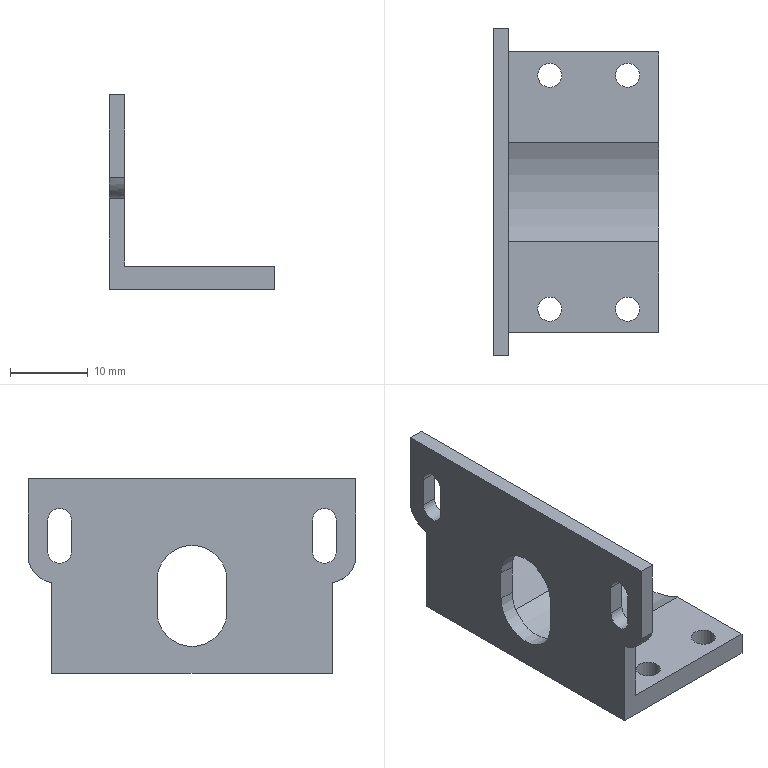Part | STEP file | Wytnij-wyci_gni_cie6_2 | 1 solid | 30 faces | box 21.259 x 42 x 25 mm | volume 3415 mm3 | plane 17 | cylinder 11 | spline 2 | commonest cylinder face diameters 3.05 x4 3.1 x4 8.97 x2 28.3 x1